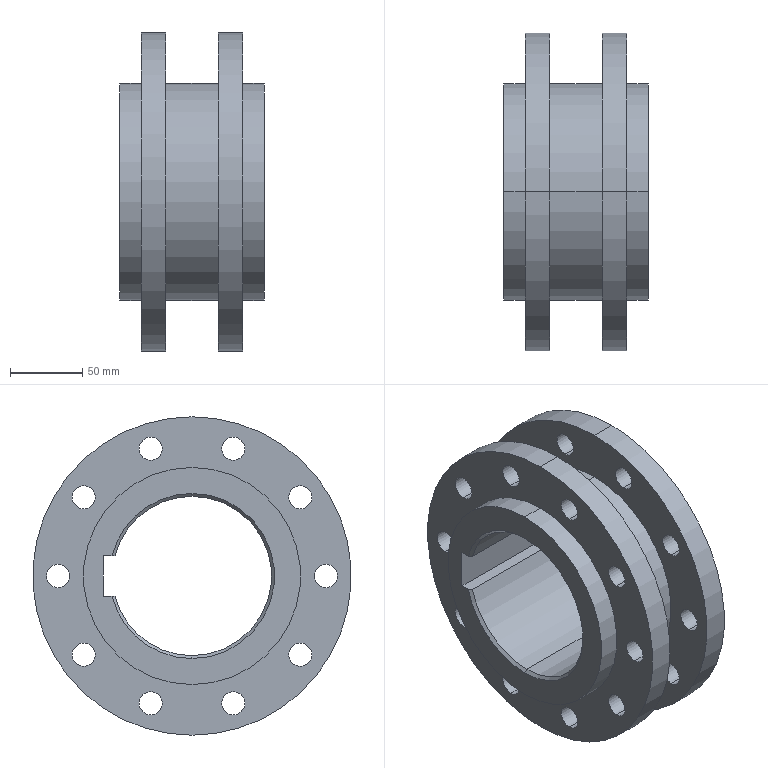Part | SolidWorks | features ICE 2, CirPattern 1, Revolution 1 | 1 solid | 68 faces | box 100 x 220 x 220 mm | volume 1419189 mm3 | cylinder 53 | plane 9 | cone 6 | commonest cylinder face diameters 16 x40 150 x6 220 x4 110 x3